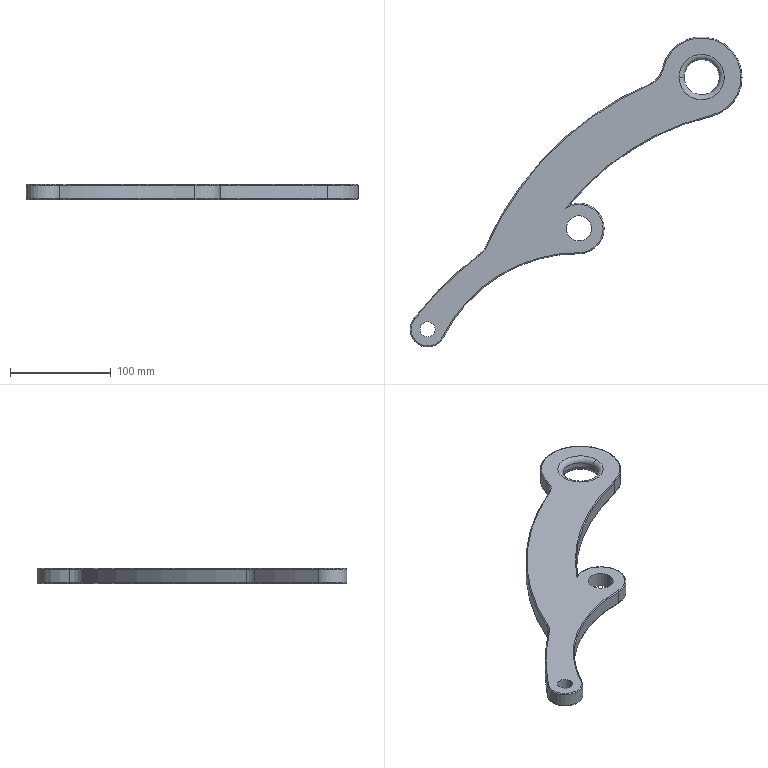Part | SolidWorks | features Fillet 3, HoleWzd 3, Extrusion 1 | 1 solid | 45 faces | box 329.193 x 307.5 x 15 mm | volume 313638 mm3 | torus 26 | cylinder 17 | plane 2 | commonest cylinder face diameters 35 x3 15 x2 25 x2 40 x2 50 x2 80 x2
STEP:
#1=CARTESIAN_POINT('',(254.193,250.,5.));
#2=VERTEX_POINT('',#1);
#3=CARTESIAN_POINT('',(289.193,250.,5.));
#4=VERTEX_POINT('',#3);
#5=CARTESIAN_POINT('',(271.693,250.,5.));
#6=DIRECTION('',(0.,0.,-1.));
#7=DIRECTION('',(1.,0.,0.));
#8=AXIS2_PLACEMENT_3D('',#5,#6,#7);
#9=CIRCLE('',#8,17.5);
#10=EDGE_CURVE('',#2,#4,#9,.T.);
#11=ORIENTED_EDGE('',*,*,#10,.F.);
#12=CARTESIAN_POINT('',(249.193,250.,0.));
#13=VERTEX_POINT('',#12);
#14=CARTESIAN_POINT('',(249.193,250.,5.));
#15=DIRECTION('',(0.,1.,0.));
#16=DIRECTION('',(-1.,0.,0.));
#17=AXIS2_PLACEMENT_3D('',#14,#15,#16);
#18=CIRCLE('',#17,5.);
#19=EDGE_CURVE('',#2,#13,#18,.T.);
#20=ORIENTED_EDGE('',*,*,#19,.T.);
#21=CARTESIAN_POINT('',(294.193,250.,0.));
#22=VERTEX_POINT('',#21);
#23=CARTESIAN_POINT('',(271.693,250.,0.));
#24=DIRECTION('',(0.,0.,1.));
#25=DIRECTION('',(1.,0.,0.));
#26=AXIS2_PLACEMENT_3D('',#23,#24,#25);
#27=CIRCLE('',#26,22.5);
#28=EDGE_CURVE('',#22,#13,#27,.T.);
#29=ORIENTED_EDGE('',*,*,#28,.F.);
#30=CARTESIAN_POINT('',(294.193,250.,5.));
#31=DIRECTION('',(0.,-1.,0.));
#32=DIRECTION('',(0.,0.,-1.));
#33=AXIS2_PLACEMENT_3D('',#30,#31,#32);
#34=CIRCLE('',#33,5.);
#35=EDGE_CURVE('',#4,#22,#34,.T.);
#36=ORIENTED_EDGE('',*,*,#35,.F.);
#37=EDGE_LOOP('',(#11,#20,#29,#36));
#38=FACE_OUTER_BOUND('',#37,.T.);
#39=CARTESIAN_POINT('',(271.693,250.,5.));
#40=DIRECTION('',(0.,0.,1.));
#41=DIRECTION('',(1.,0.,0.));
#42=AXIS2_PLACEMENT_3D('',#39,#40,#41);
#43=TOROIDAL_SURFACE('',#42,22.5,5.);
#44=ADVANCED_FACE('',(#38),#43,.T.);
#45=CARTESIAN_POINT('',(249.193,250.,15.));
#46=VERTEX_POINT('',#45);
#47=CARTESIAN_POINT('',(294.193,250.,15.));
#48=VERTEX_POINT('',#47);
#49=CARTESIAN_POINT('',(271.693,250.,15.));
#50=DIRECTION('',(0.,0.,-1.));
#51=DIRECTION('',(1.,0.,0.));
#52=AXIS2_PLACEMENT_3D('',#49,#50,#51);
#53=CIRCLE('',#52,22.5);
#54=EDGE_CURVE('',#46,#48,#53,.T.);
#55=ORIENTED_EDGE('',*,*,#54,.F.);
#56=CARTESIAN_POINT('',(254.193,250.,10.));
#57=VERTEX_POINT('',#56);
#58=CARTESIAN_POINT('',(249.193,250.,10.));
#59=DIRECTION('',(0.,1.,0.));
#60=DIRECTION('',(-1.,0.,0.));
#61=AXIS2_PLACEMENT_3D('',#58,#59,#60);
#62=CIRCLE('',#61,5.);
#63=EDGE_CURVE('',#46,#57,#62,.T.);
#64=ORIENTED_EDGE('',*,*,#63,.T.);
#65=CARTESIAN_POINT('',(289.193,250.,10.));
#66=VERTEX_POINT('',#65);
#67=CARTESIAN_POINT('',(271.693,250.,10.));
#68=DIRECTION('',(0.,0.,1.));
#69=DIRECTION('',(1.,0.,0.));
#70=AXIS2_PLACEMENT_3D('',#67,#68,#69);
#71=CIRCLE('',#70,17.5);
#72=EDGE_CURVE('',#66,#57,#71,.T.);
#73=ORIENTED_EDGE('',*,*,#72,.F.);
#74=CARTESIAN_POINT('',(294.193,250.,10.));
#75=DIRECTION('',(0.,-1.,0.));
#76=DIRECTION('',(0.,0.,-1.));
#77=AXIS2_PLACEMENT_3D('',#74,#75,#76);
#78=CIRCLE('',#77,5.);
#79=EDGE_CURVE('',#48,#66,#78,.T.);
#80=ORIENTED_EDGE('',*,*,#79,.F.);
#81=EDGE_LOOP('',(#55,#64,#73,#80));
#82=FACE_OUTER_BOUND('',#81,.T.);
#83=CARTESIAN_POINT('',(271.693,250.,10.));
#84=DIRECTION('',(0.,0.,1.));
#85=DIRECTION('',(1.,0.,0.));
#86=AXIS2_PLACEMENT_3D('',#83,#84,#85);
#87=TOROIDAL_SURFACE('',#86,22.5,5.);
#88=ADVANCED_FACE('',(#82),#87,.T.);
#89=CARTESIAN_POINT('',(311.693,250.,14.));
#90=VERTEX_POINT('',#89);
#91=CARTESIAN_POINT('',(281.029,211.105,14.));
#92=VERTEX_POINT('',#91);
#93=CARTESIAN_POINT('',(271.693,250.,14.));
#94=DIRECTION('',(0.,0.,-1.));
#95=DIRECTION('',(1.,0.,0.));
#96=AXIS2_PLACEMENT_3D('',#93,#94,#95);
#97=CIRCLE('',#96,40.);
#98=EDGE_CURVE('',#90,#92,#97,.T.);
#99=ORIENTED_EDGE('',*,*,#98,.F.);
#100=CARTESIAN_POINT('',(310.693,250.,15.));
#101=VERTEX_POINT('',#100);
#102=CARTESIAN_POINT('',(310.693,250.,14.));
#103=DIRECTION('',(0.,-1.,0.));
#104=DIRECTION('',(0.,0.,-1.));
#105=AXIS2_PLACEMENT_3D('',#102,#103,#104);
#106=CIRCLE('',#105,1.);
#107=EDGE_CURVE('',#90,#101,#106,.T.);
#108=ORIENTED_EDGE('',*,*,#107,.T.);
#109=CARTESIAN_POINT('',(280.795,212.077,15.));
#110=VERTEX_POINT('',#109);
#111=CARTESIAN_POINT('',(271.693,250.,15.));
#112=DIRECTION('',(0.,0.,1.));
#113=DIRECTION('',(1.,0.,0.));
#114=AXIS2_PLACEMENT_3D('',#111,#112,#113);
#115=CIRCLE('',#114,39.);
#116=EDGE_CURVE('',#110,#101,#115,.T.);
#117=ORIENTED_EDGE('',*,*,#116,.F.);
#118=CARTESIAN_POINT('',(280.795,212.077,14.));
#119=DIRECTION('',(-0.9724,-0.2334,0.));
#120=DIRECTION('',(0.2334,-0.9724,0.));
#121=AXIS2_PLACEMENT_3D('',#118,#119,#120);
#122=CIRCLE('',#121,1.);
#123=EDGE_CURVE('',#92,#110,#122,.T.);
#124=ORIENTED_EDGE('',*,*,#123,.F.);
#125=EDGE_LOOP('',(#99,#108,#117,#124));
#126=FACE_OUTER_BOUND('',#125,.T.);
#127=CARTESIAN_POINT('',(271.693,250.,14.));
#128=DIRECTION('',(0.,0.,1.));
#129=DIRECTION('',(1.,0.,0.));
#130=AXIS2_PLACEMENT_3D('',#127,#128,#129);
#131=TOROIDAL_SURFACE('',#130,39.,1.);
#132=ADVANCED_FACE('',(#126),#131,.T.);
#133=CARTESIAN_POINT('',(175.,100.,14.));
#134=VERTEX_POINT('',#133);
#135=CARTESIAN_POINT('',(149.967,75.,14.));
#136=VERTEX_POINT('',#135);
#137=CARTESIAN_POINT('',(150.,100.,14.));
#138=DIRECTION('',(0.,0.,-1.));
#139=DIRECTION('',(1.,0.,0.));
#140=AXIS2_PLACEMENT_3D('',#137,#138,#139);
#141=CIRCLE('',#140,25.);
#142=EDGE_CURVE('',#134,#136,#141,.T.);
#143=ORIENTED_EDGE('',*,*,#142,.F.);
#144=CARTESIAN_POINT('',(174.,100.,15.));
#145=VERTEX_POINT('',#144);
#146=CARTESIAN_POINT('',(174.,100.,14.));
#147=DIRECTION('',(0.,-1.,0.));
#148=DIRECTION('',(0.,0.,-1.));
#149=AXIS2_PLACEMENT_3D('',#146,#147,#148);
#150=CIRCLE('',#149,1.);
#151=EDGE_CURVE('',#134,#145,#150,.T.);
#152=ORIENTED_EDGE('',*,*,#151,.T.);
#153=CARTESIAN_POINT('',(149.969,76.,15.));
#154=VERTEX_POINT('',#153);
#155=CARTESIAN_POINT('',(150.,100.,15.));
#156=DIRECTION('',(0.,0.,1.));
#157=DIRECTION('',(1.,0.,0.));
#158=AXIS2_PLACEMENT_3D('',#155,#156,#157);
#159=CIRCLE('',#158,24.);
#160=EDGE_CURVE('',#154,#145,#159,.T.);
#161=ORIENTED_EDGE('',*,*,#160,.F.);
#162=CARTESIAN_POINT('',(149.969,76.,14.));
#163=DIRECTION('',(1.,-0.00131,0.));
#164=DIRECTION('',(0.00131,1.,0.));
#165=AXIS2_PLACEMENT_3D('',#162,#163,#164);
#166=CIRCLE('',#165,1.);
#167=EDGE_CURVE('',#154,#136,#166,.T.);
#168=ORIENTED_EDGE('',*,*,#167,.T.);
#169=EDGE_LOOP('',(#143,#152,#161,#168));
#170=FACE_OUTER_BOUND('',#169,.T.);
#171=CARTESIAN_POINT('',(150.,100.,14.));
#172=DIRECTION('',(0.,0.,1.));
#173=DIRECTION('',(1.,0.,0.));
#174=AXIS2_PLACEMENT_3D('',#171,#172,#173);
#175=TOROIDAL_SURFACE('',#174,24.,1.);
#176=ADVANCED_FACE('',(#170),#175,.T.);
#177=CARTESIAN_POINT('',(310.693,250.,0.));
#178=VERTEX_POINT('',#177);
#179=CARTESIAN_POINT('',(280.795,212.077,0.));
#180=VERTEX_POINT('',#179);
#181=CARTESIAN_POINT('',(271.693,250.,0.));
#182=DIRECTION('',(0.,0.,-1.));
#183=DIRECTION('',(1.,0.,0.));
#184=AXIS2_PLACEMENT_3D('',#181,#182,#183);
#185=CIRCLE('',#184,39.);
#186=EDGE_CURVE('',#178,#180,#185,.T.);
#187=ORIENTED_EDGE('',*,*,#186,.F.);
#188=CARTESIAN_POINT('',(311.693,250.,1.));
#189=VERTEX_POINT('',#188);
#190=CARTESIAN_POINT('',(310.693,250.,1.));
#191=DIRECTION('',(0.,-1.,0.));
#192=DIRECTION('',(0.,0.,-1.));
#193=AXIS2_PLACEMENT_3D('',#190,#191,#192);
#194=CIRCLE('',#193,1.);
#195=EDGE_CURVE('',#178,#189,#194,.T.);
#196=ORIENTED_EDGE('',*,*,#195,.T.);
#197=CARTESIAN_POINT('',(281.029,211.105,1.));
#198=VERTEX_POINT('',#197);
#199=CARTESIAN_POINT('',(271.693,250.,1.));
#200=DIRECTION('',(0.,0.,1.));
#201=DIRECTION('',(1.,0.,0.));
#202=AXIS2_PLACEMENT_3D('',#199,#200,#201);
#203=CIRCLE('',#202,40.);
#204=EDGE_CURVE('',#198,#189,#203,.T.);
#205=ORIENTED_EDGE('',*,*,#204,.F.);
#206=CARTESIAN_POINT('',(280.795,212.077,1.));
#207=DIRECTION('',(-0.9724,-0.2334,0.));
#208=DIRECTION('',(0.2334,-0.9724,0.));
#209=AXIS2_PLACEMENT_3D('',#206,#207,#208);
#210=CIRCLE('',#209,1.);
#211=EDGE_CURVE('',#180,#198,#210,.T.);
#212=ORIENTED_EDGE('',*,*,#211,.F.);
#213=EDGE_LOOP('',(#187,#196,#205,#212));
#214=FACE_OUTER_BOUND('',#213,.T.);
#215=CARTESIAN_POINT('',(271.693,250.,1.));
#216=DIRECTION('',(0.,0.,1.));
#217=DIRECTION('',(1.,0.,0.));
#218=AXIS2_PLACEMENT_3D('',#215,#216,#217);
#219=TOROIDAL_SURFACE('',#218,39.,1.);
#220=ADVANCED_FACE('',(#214),#219,.T.);
#221=CARTESIAN_POINT('',(174.,100.,0.));
#222=VERTEX_POINT('',#221);
#223=CARTESIAN_POINT('',(149.969,76.,0.));
#224=VERTEX_POINT('',#223);
#225=CARTESIAN_POINT('',(150.,100.,0.));
#226=DIRECTION('',(0.,0.,-1.));
#227=DIRECTION('',(1.,0.,0.));
#228=AXIS2_PLACEMENT_3D('',#225,#226,#227);
#229=CIRCLE('',#228,24.);
#230=EDGE_CURVE('',#222,#224,#229,.T.);
#231=ORIENTED_EDGE('',*,*,#230,.F.);
#232=CARTESIAN_POINT('',(175.,100.,1.));
#233=VERTEX_POINT('',#232);
#234=CARTESIAN_POINT('',(174.,100.,1.));
#235=DIRECTION('',(0.,-1.,0.));
#236=DIRECTION('',(0.,0.,-1.));
#237=AXIS2_PLACEMENT_3D('',#234,#235,#236);
#238=CIRCLE('',#237,1.);
#239=EDGE_CURVE('',#222,#233,#238,.T.);
#240=ORIENTED_EDGE('',*,*,#239,.T.);
#241=CARTESIAN_POINT('',(149.967,75.,1.));
#242=VERTEX_POINT('',#241);
#243=CARTESIAN_POINT('',(150.,100.,1.));
#244=DIRECTION('',(0.,0.,1.));
#245=DIRECTION('',(1.,0.,0.));
#246=AXIS2_PLACEMENT_3D('',#243,#244,#245);
#247=CIRCLE('',#246,25.);
#248=EDGE_CURVE('',#242,#233,#247,.T.);
#249=ORIENTED_EDGE('',*,*,#248,.F.);
#250=CARTESIAN_POINT('',(149.969,76.,1.));
#251=DIRECTION('',(1.,-0.00131,0.));
#252=DIRECTION('',(0.00131,1.,0.));
#253=AXIS2_PLACEMENT_3D('',#250,#251,#252);
#254=CIRCLE('',#253,1.);
#255=EDGE_CURVE('',#242,#224,#254,.T.);
#256=ORIENTED_EDGE('',*,*,#255,.T.);
#257=EDGE_LOOP('',(#231,#240,#249,#256));
#258=FACE_OUTER_BOUND('',#257,.T.);
#259=CARTESIAN_POINT('',(150.,100.,1.));
#260=DIRECTION('',(0.,0.,1.));
#261=DIRECTION('',(1.,0.,0.));
#262=AXIS2_PLACEMENT_3D('',#259,#260,#261);
#263=TOROIDAL_SURFACE('',#262,24.,1.);
#264=ADVANCED_FACE('',(#258),#263,.T.);
#265=CARTESIAN_POINT('',(7.5,0.,15.));
#266=VERTEX_POINT('',#265);
#267=CARTESIAN_POINT('',(-7.5,0.,15.));
#268=VERTEX_POINT('',#267);
#269=CARTESIAN_POINT('',(0.,0.,15.));
#270=DIRECTION('',(0.,0.,-1.));
#271=DIRECTION('',(-1.,0.,0.));
#272=AXIS2_PLACEMENT_3D('',#269,#270,#271);
#273=CIRCLE('',#272,7.5);
#274=EDGE_CURVE('',#266,#268,#273,.T.);
#275=ORIENTED_EDGE('',*,*,#274,.F.);
#276=CARTESIAN_POINT('',(7.5,0.,0.));
#277=VERTEX_POINT('',#276);
#278=CARTESIAN_POINT('',(7.5,0.,0.));
#279=DIRECTION('',(0.,0.,-1.));
#280=VECTOR('',#279,1000.);
#281=LINE('',#278,#280);
#282=EDGE_CURVE('',#266,#277,#281,.T.);
#283=ORIENTED_EDGE('',*,*,#282,.T.);
#284=CARTESIAN_POINT('',(-7.5,0.,0.));
#285=VERTEX_POINT('',#284);
#286=CARTESIAN_POINT('',(0.,0.,0.));
#287=DIRECTION('',(0.,0.,-1.));
#288=DIRECTION('',(-1.,0.,0.));
#289=AXIS2_PLACEMENT_3D('',#286,#287,#288);
#290=CIRCLE('',#289,7.5);
#291=EDGE_CURVE('',#277,#285,#290,.T.);
#292=ORIENTED_EDGE('',*,*,#291,.T.);
#293=CARTESIAN_POINT('',(-7.5,0.,0.));
#294=DIRECTION('',(0.,0.,-1.));
#295=VECTOR('',#294,1000.);
#296=LINE('',#293,#295);
#297=EDGE_CURVE('',#268,#285,#296,.T.);
#298=ORIENTED_EDGE('',*,*,#297,.F.);
#299=EDGE_LOOP('',(#275,#283,#292,#298));
#300=FACE_OUTER_BOUND('',#299,.T.);
#301=CARTESIAN_POINT('',(0.,0.,0.));
#302=DIRECTION('',(0.,0.,-1.));
#303=DIRECTION('',(-1.,0.,0.));
#304=AXIS2_PLACEMENT_3D('',#301,#302,#303);
#305=CYLINDRICAL_SURFACE('',#304,7.5);
#306=ADVANCED_FACE('',(#300),#305,.F.);
#307=CARTESIAN_POINT('',(162.5,100.,15.));
#308=VERTEX_POINT('',#307);
#309=CARTESIAN_POINT('',(137.5,100.,15.));
#310=VERTEX_POINT('',#309);
#311=CARTESIAN_POINT('',(150.,100.,15.));
#312=DIRECTION('',(0.,0.,-1.));
#313=DIRECTION('',(-1.,0.,0.));
#314=AXIS2_PLACEMENT_3D('',#311,#312,#313);
#315=CIRCLE('',#314,12.5);
#316=EDGE_CURVE('',#308,#310,#315,.T.);
#317=ORIENTED_EDGE('',*,*,#316,.F.);
#318=CARTESIAN_POINT('',(162.5,100.,0.));
#319=VERTEX_POINT('',#318);
#320=CARTESIAN_POINT('',(162.5,100.,0.));
#321=DIRECTION('',(0.,0.,-1.));
#322=VECTOR('',#321,1000.);
#323=LINE('',#320,#322);
#324=EDGE_CURVE('',#308,#319,#323,.T.);
#325=ORIENTED_EDGE('',*,*,#324,.T.);
#326=CARTESIAN_POINT('',(137.5,100.,0.));
#327=VERTEX_POINT('',#326);
#328=CARTESIAN_POINT('',(150.,100.,0.));
#329=DIRECTION('',(0.,0.,-1.));
#330=DIRECTION('',(-1.,0.,0.));
#331=AXIS2_PLACEMENT_3D('',#328,#329,#330);
#332=CIRCLE('',#331,12.5);
#333=EDGE_CURVE('',#319,#327,#332,.T.);
#334=ORIENTED_EDGE('',*,*,#333,.T.);
#335=CARTESIAN_POINT('',(137.5,100.,0.));
#336=DIRECTION('',(0.,0.,-1.));
#337=VECTOR('',#336,1000.);
#338=LINE('',#335,#337);
#339=EDGE_CURVE('',#310,#327,#338,.T.);
#340=ORIENTED_EDGE('',*,*,#339,.F.);
#341=EDGE_LOOP('',(#317,#325,#334,#340));
#342=FACE_OUTER_BOUND('',#341,.T.);
#343=CARTESIAN_POINT('',(150.,100.,0.));
#344=DIRECTION('',(0.,0.,-1.));
#345=DIRECTION('',(-1.,0.,0.));
#346=AXIS2_PLACEMENT_3D('',#343,#344,#345);
#347=CYLINDRICAL_SURFACE('',#346,12.5);
#348=ADVANCED_FACE('',(#342),#347,.F.);
#349=CARTESIAN_POINT('',(271.693,250.,10.));
#350=DIRECTION('',(0.,0.,1.));
#351=DIRECTION('',(1.,0.,0.));
#352=AXIS2_PLACEMENT_3D('',#349,#350,#351);
#353=CIRCLE('',#352,17.5);
#354=EDGE_CURVE('',#57,#66,#353,.T.);
#355=ORIENTED_EDGE('',*,*,#354,.T.);
#356=CARTESIAN_POINT('',(289.193,250.,0.));
#357=DIRECTION('',(0.,0.,-1.));
#358=VECTOR('',#357,1000.);
#359=LINE('',#356,#358);
#360=EDGE_CURVE('',#66,#4,#359,.T.);
#361=ORIENTED_EDGE('',*,*,#360,.T.);
#362=CARTESIAN_POINT('',(271.693,250.,5.));
#363=DIRECTION('',(0.,0.,-1.));
#364=DIRECTION('',(1.,0.,0.));
#365=AXIS2_PLACEMENT_3D('',#362,#363,#364);
#366=CIRCLE('',#365,17.5);
#367=EDGE_CURVE('',#4,#2,#366,.T.);
#368=ORIENTED_EDGE('',*,*,#367,.T.);
#369=CARTESIAN_POINT('',(254.193,250.,0.));
#370=DIRECTION('',(0.,0.,-1.));
#371=VECTOR('',#370,1000.);
#372=LINE('',#369,#371);
#373=EDGE_CURVE('',#57,#2,#372,.T.);
#374=ORIENTED_EDGE('',*,*,#373,.F.);
#375=EDGE_LOOP('',(#355,#361,#368,#374));
#376=FACE_OUTER_BOUND('',#375,.T.);
#377=CARTESIAN_POINT('',(271.693,250.,0.));
#378=DIRECTION('',(0.,0.,-1.));
#379=DIRECTION('',(-1.,0.,0.));
#380=AXIS2_PLACEMENT_3D('',#377,#378,#379);
#381=CYLINDRICAL_SURFACE('',#380,17.5);
#382=ADVANCED_FACE('',(#376),#381,.F.);
#383=ORIENTED_EDGE('',*,*,#248,.T.);
#384=CARTESIAN_POINT('',(175.,100.,0.));
#385=DIRECTION('',(0.,0.,1.));
#386=VECTOR('',#385,1000.);
#387=LINE('',#384,#386);
#388=EDGE_CURVE('',#233,#134,#387,.T.);
#389=ORIENTED_EDGE('',*,*,#388,.T.);
#390=ORIENTED_EDGE('',*,*,#142,.T.);
#391=CARTESIAN_POINT('',(149.967,75.,0.));
#392=DIRECTION('',(0.,0.,1.));
#393=VECTOR('',#392,1000.);
#394=LINE('',#391,#393);
#395=EDGE_CURVE('',#242,#136,#394,.T.);
#396=ORIENTED_EDGE('',*,*,#395,.F.);
#397=EDGE_LOOP('',(#383,#389,#390,#396));
#398=FACE_OUTER_BOUND('',#397,.T.);
#399=CARTESIAN_POINT('',(150.,100.,0.));
#400=DIRECTION('',(0.,0.,1.));
#401=DIRECTION('',(1.,0.,0.));
#402=AXIS2_PLACEMENT_3D('',#399,#400,#401);
#403=CYLINDRICAL_SURFACE('',#402,25.);
#404=ADVANCED_FACE('',(#398),#403,.T.);
#405=ORIENTED_EDGE('',*,*,#204,.T.);
#406=CARTESIAN_POINT('',(311.693,250.,0.));
#407=DIRECTION('',(0.,0.,1.));
#408=VECTOR('',#407,1000.);
#409=LINE('',#406,#408);
#410=EDGE_CURVE('',#189,#90,#409,.T.);
#411=ORIENTED_EDGE('',*,*,#410,.T.);
#412=ORIENTED_EDGE('',*,*,#98,.T.);
#413=CARTESIAN_POINT('',(281.029,211.105,0.));
#414=DIRECTION('',(0.,0.,1.));
#415=VECTOR('',#414,1000.);
#416=LINE('',#413,#415);
#417=EDGE_CURVE('',#198,#92,#416,.T.);
#418=ORIENTED_EDGE('',*,*,#417,.F.);
#419=EDGE_LOOP('',(#405,#411,#412,#418));
#420=FACE_OUTER_BOUND('',#419,.T.);
#421=CARTESIAN_POINT('',(271.693,250.,0.));
#422=DIRECTION('',(0.,0.,1.));
#423=DIRECTION('',(1.,0.,0.));
#424=AXIS2_PLACEMENT_3D('',#421,#422,#423);
#425=CYLINDRICAL_SURFACE('',#424,40.);
#426=ADVANCED_FACE('',(#420),#425,.T.);
#427=ORIENTED_EDGE('',*,*,#410,.F.);
#428=CARTESIAN_POINT('',(232.517,258.08,1.));
#429=VERTEX_POINT('',#428);
#430=CARTESIAN_POINT('',(271.693,250.,1.));
#431=DIRECTION('',(0.,0.,1.));
#432=DIRECTION('',(1.,0.,0.));
#433=AXIS2_PLACEMENT_3D('',#430,#431,#432);
#434=CIRCLE('',#433,40.);
#435=EDGE_CURVE('',#189,#429,#434,.T.);
#436=ORIENTED_EDGE('',*,*,#435,.T.);
#437=CARTESIAN_POINT('',(232.517,258.08,14.));
#438=VERTEX_POINT('',#437);
#439=CARTESIAN_POINT('',(232.517,258.08,0.));
#440=DIRECTION('',(0.,0.,1.));
#441=VECTOR('',#440,1000.);
#442=LINE('',#439,#441);
#443=EDGE_CURVE('',#429,#438,#442,.T.);
#444=ORIENTED_EDGE('',*,*,#443,.T.);
#445=CARTESIAN_POINT('',(271.693,250.,14.));
#446=DIRECTION('',(0.,0.,-1.));
#447=DIRECTION('',(1.,0.,0.));
#448=AXIS2_PLACEMENT_3D('',#445,#446,#447);
#449=CIRCLE('',#448,40.);
#450=EDGE_CURVE('',#438,#90,#449,.T.);
#451=ORIENTED_EDGE('',*,*,#450,.T.);
#452=EDGE_LOOP('',(#427,#436,#444,#451));
#453=FACE_OUTER_BOUND('',#452,.T.);
#454=CARTESIAN_POINT('',(271.693,250.,0.));
#455=DIRECTION('',(0.,0.,1.));
#456=DIRECTION('',(1.,0.,0.));
#457=AXIS2_PLACEMENT_3D('',#454,#455,#456);
#458=CYLINDRICAL_SURFACE('',#457,40.);
#459=ADVANCED_FACE('',(#453),#458,.T.);
#460=CARTESIAN_POINT('',(140.715,123.212,1.));
#461=VERTEX_POINT('',#460);
#462=CARTESIAN_POINT('',(140.715,123.212,14.));
#463=VERTEX_POINT('',#462);
#464=CARTESIAN_POINT('',(140.715,123.212,0.));
#465=DIRECTION('',(0.,0.,1.));
#466=VECTOR('',#465,1000.);
#467=LINE('',#464,#466);
#468=EDGE_CURVE('',#461,#463,#467,.T.);
#469=ORIENTED_EDGE('',*,*,#468,.F.);
#470=CARTESIAN_POINT('',(341.711,-41.715,1.));
#471=DIRECTION('',(0.,0.,-1.));
#472=DIRECTION('',(1.,0.,0.));
#473=AXIS2_PLACEMENT_3D('',#470,#471,#472);
#474=CIRCLE('',#473,260.);
#475=EDGE_CURVE('',#461,#198,#474,.T.);
#476=ORIENTED_EDGE('',*,*,#475,.T.);
#477=ORIENTED_EDGE('',*,*,#417,.T.);
#478=CARTESIAN_POINT('',(341.711,-41.715,14.));
#479=DIRECTION('',(0.,0.,1.));
#480=DIRECTION('',(1.,0.,0.));
#481=AXIS2_PLACEMENT_3D('',#478,#479,#480);
#482=CIRCLE('',#481,260.);
#483=EDGE_CURVE('',#92,#463,#482,.T.);
#484=ORIENTED_EDGE('',*,*,#483,.T.);
#485=EDGE_LOOP('',(#469,#476,#477,#484));
#486=FACE_OUTER_BOUND('',#485,.T.);
#487=CARTESIAN_POINT('',(341.711,-41.715,0.));
#488=DIRECTION('',(0.,0.,1.));
#489=DIRECTION('',(1.,0.,0.));
#490=AXIS2_PLACEMENT_3D('',#487,#488,#489);
#491=CYLINDRICAL_SURFACE('',#490,260.);
#492=ADVANCED_FACE('',(#486),#491,.F.);
#493=ORIENTED_EDGE('',*,*,#388,.F.);
#494=CARTESIAN_POINT('',(150.,100.,1.));
#495=DIRECTION('',(0.,0.,1.));
#496=DIRECTION('',(1.,0.,0.));
#497=AXIS2_PLACEMENT_3D('',#494,#495,#496);
#498=CIRCLE('',#497,25.);
#499=EDGE_CURVE('',#233,#461,#498,.T.);
#500=ORIENTED_EDGE('',*,*,#499,.T.);
#501=ORIENTED_EDGE('',*,*,#468,.T.);
#502=CARTESIAN_POINT('',(150.,100.,14.));
#503=DIRECTION('',(0.,0.,-1.));
#504=DIRECTION('',(1.,0.,0.));
#505=AXIS2_PLACEMENT_3D('',#502,#503,#504);
#506=CIRCLE('',#505,25.);
#507=EDGE_CURVE('',#463,#134,#506,.T.);
#508=ORIENTED_EDGE('',*,*,#507,.T.);
#509=EDGE_LOOP('',(#493,#500,#501,#508));
#510=FACE_OUTER_BOUND('',#509,.T.);
#511=CARTESIAN_POINT('',(150.,100.,0.));
#512=DIRECTION('',(0.,0.,1.));
#513=DIRECTION('',(1.,0.,0.));
#514=AXIS2_PLACEMENT_3D('',#511,#512,#513);
#515=CYLINDRICAL_SURFACE('',#514,25.);
#516=ADVANCED_FACE('',(#510),#515,.T.);
#517=CARTESIAN_POINT('',(15.648,-7.836,1.));
#518=VERTEX_POINT('',#517);
#519=CARTESIAN_POINT('',(15.648,-7.836,14.));
#520=VERTEX_POINT('',#519);
#521=CARTESIAN_POINT('',(15.648,-7.836,0.));
#522=DIRECTION('',(0.,0.,1.));
#523=VECTOR('',#522,1000.);
#524=LINE('',#521,#523);
#525=EDGE_CURVE('',#518,#520,#524,.T.);
#526=ORIENTED_EDGE('',*,*,#525,.F.);
#527=CARTESIAN_POINT('',(149.771,-75.,1.));
#528=DIRECTION('',(0.,0.,-1.));
#529=DIRECTION('',(1.,0.,0.));
#530=AXIS2_PLACEMENT_3D('',#527,#528,#529);
#531=CIRCLE('',#530,150.);
#532=EDGE_CURVE('',#518,#242,#531,.T.);
#533=ORIENTED_EDGE('',*,*,#532,.T.);
#534=ORIENTED_EDGE('',*,*,#395,.T.);
#535=CARTESIAN_POINT('',(149.771,-75.,14.));
#536=DIRECTION('',(0.,0.,1.));
#537=DIRECTION('',(1.,0.,0.));
#538=AXIS2_PLACEMENT_3D('',#535,#536,#537);
#539=CIRCLE('',#538,150.);
#540=EDGE_CURVE('',#136,#520,#539,.T.);
#541=ORIENTED_EDGE('',*,*,#540,.T.);
#542=EDGE_LOOP('',(#526,#533,#534,#541));
#543=FACE_OUTER_BOUND('',#542,.T.);
#544=CARTESIAN_POINT('',(149.771,-75.,0.));
#545=DIRECTION('',(0.,0.,1.));
#546=DIRECTION('',(1.,0.,0.));
#547=AXIS2_PLACEMENT_3D('',#544,#545,#546);
#548=CYLINDRICAL_SURFACE('',#547,150.);
#549=ADVANCED_FACE('',(#543),#548,.F.);
#550=CARTESIAN_POINT('',(-13.768,10.803,1.));
#551=VERTEX_POINT('',#550);
#552=CARTESIAN_POINT('',(-13.768,10.803,14.));
#553=VERTEX_POINT('',#552);
#554=CARTESIAN_POINT('',(-13.768,10.803,0.));
#555=DIRECTION('',(0.,0.,1.));
#556=VECTOR('',#555,1000.);
#557=LINE('',#554,#556);
#558=EDGE_CURVE('',#551,#553,#557,.T.);
#559=ORIENTED_EDGE('',*,*,#558,.F.);
#560=CARTESIAN_POINT('',(0.,0.,1.));
#561=DIRECTION('',(0.,0.,1.));
#562=DIRECTION('',(1.,0.,0.));
#563=AXIS2_PLACEMENT_3D('',#560,#561,#562);
#564=CIRCLE('',#563,17.5);
#565=EDGE_CURVE('',#551,#518,#564,.T.);
#566=ORIENTED_EDGE('',*,*,#565,.T.);
#567=ORIENTED_EDGE('',*,*,#525,.T.);
#568=CARTESIAN_POINT('',(0.,0.,14.));
#569=DIRECTION('',(0.,0.,-1.));
#570=DIRECTION('',(1.,0.,0.));
#571=AXIS2_PLACEMENT_3D('',#568,#569,#570);
#572=CIRCLE('',#571,17.5);
#573=EDGE_CURVE('',#520,#553,#572,.T.);
#574=ORIENTED_EDGE('',*,*,#573,.T.);
#575=EDGE_LOOP('',(#559,#566,#567,#574));
#576=FACE_OUTER_BOUND('',#575,.T.);
#577=CARTESIAN_POINT('',(0.,0.,0.));
#578=DIRECTION('',(0.,0.,1.));
#579=DIRECTION('',(1.,0.,0.));
#580=AXIS2_PLACEMENT_3D('',#577,#578,#579);
#581=CYLINDRICAL_SURFACE('',#580,17.5);
#582=ADVANCED_FACE('',(#576),#581,.T.);
#583=CARTESIAN_POINT('',(51.411,74.615,14.));
#584=VERTEX_POINT('',#583);
#585=CARTESIAN_POINT('',(51.411,74.615,1.));
#586=VERTEX_POINT('',#585);
#587=CARTESIAN_POINT('',(51.411,74.615,0.));
#588=DIRECTION('',(0.,0.,-1.));
#589=VECTOR('',#588,1000.);
#590=LINE('',#587,#589);
#591=EDGE_CURVE('',#584,#586,#590,.T.);
#592=ORIENTED_EDGE('',*,*,#591,.T.);
#593=CARTESIAN_POINT('',(261.585,-205.255,1.));
#594=DIRECTION('',(0.,0.,1.));
#595=DIRECTION('',(1.,0.,0.));
#596=AXIS2_PLACEMENT_3D('',#593,#594,#595);
#597=CIRCLE('',#596,350.);
#598=EDGE_CURVE('',#586,#551,#597,.T.);
#599=ORIENTED_EDGE('',*,*,#598,.T.);
#600=ORIENTED_EDGE('',*,*,#558,.T.);
#601=CARTESIAN_POINT('',(261.585,-205.255,14.));
#602=DIRECTION('',(0.,0.,-1.));
#603=DIRECTION('',(1.,0.,0.));
#604=AXIS2_PLACEMENT_3D('',#601,#602,#603);
#605=CIRCLE('',#604,350.);
#606=EDGE_CURVE('',#553,#584,#605,.T.);
#607=ORIENTED_EDGE('',*,*,#606,.T.);
#608=EDGE_LOOP('',(#592,#599,#600,#607));
#609=FACE_OUTER_BOUND('',#608,.T.);
#610=CARTESIAN_POINT('',(261.585,-205.255,0.));
#611=DIRECTION('',(0.,0.,1.));
#612=DIRECTION('',(1.,0.,0.));
#613=AXIS2_PLACEMENT_3D('',#610,#611,#612);
#614=CYLINDRICAL_SURFACE('',#613,350.);
#615=ADVANCED_FACE('',(#609),#614,.T.);
#616=CARTESIAN_POINT('',(220.735,243.706,14.));
#617=VERTEX_POINT('',#616);
#618=CARTESIAN_POINT('',(220.735,243.706,1.));
#619=VERTEX_POINT('',#618);
#620=CARTESIAN_POINT('',(220.735,243.706,0.));
#621=DIRECTION('',(0.,0.,-1.));
#622=VECTOR('',#621,1000.);
#623=LINE('',#620,#622);
#624=EDGE_CURVE('',#617,#619,#623,.T.);
#625=ORIENTED_EDGE('',*,*,#624,.T.);
#626=CARTESIAN_POINT('',(57.723,82.588,1.));
#627=VERTEX_POINT('',#626);
#628=CARTESIAN_POINT('',(341.711,-41.715,1.));
#629=DIRECTION('',(0.,0.,1.));
#630=DIRECTION('',(1.,0.,0.));
#631=AXIS2_PLACEMENT_3D('',#628,#629,#630);
#632=CIRCLE('',#631,310.);
#633=EDGE_CURVE('',#619,#627,#632,.T.);
#634=ORIENTED_EDGE('',*,*,#633,.T.);
#635=CARTESIAN_POINT('',(57.723,82.588,14.));
#636=VERTEX_POINT('',#635);
#637=CARTESIAN_POINT('',(57.723,82.588,0.));
#638=DIRECTION('',(0.,0.,1.));
#639=VECTOR('',#638,1000.);
#640=LINE('',#637,#639);
#641=EDGE_CURVE('',#627,#636,#640,.T.);
#642=ORIENTED_EDGE('',*,*,#641,.T.);
#643=CARTESIAN_POINT('',(341.711,-41.715,14.));
#644=DIRECTION('',(0.,0.,-1.));
#645=DIRECTION('',(1.,0.,0.));
#646=AXIS2_PLACEMENT_3D('',#643,#644,#645);
#647=CIRCLE('',#646,310.);
#648=EDGE_CURVE('',#636,#617,#647,.T.);
#649=ORIENTED_EDGE('',*,*,#648,.T.);
#650=EDGE_LOOP('',(#625,#634,#642,#649));
#651=FACE_OUTER_BOUND('',#650,.T.);
#652=CARTESIAN_POINT('',(341.711,-41.715,0.));
#653=DIRECTION('',(0.,0.,1.));
#654=DIRECTION('',(1.,0.,0.));
#655=AXIS2_PLACEMENT_3D('',#652,#653,#654);
#656=CYLINDRICAL_SURFACE('',#655,310.);
#657=ADVANCED_FACE('',(#651),#656,.T.);
#658=ORIENTED_EDGE('',*,*,#28,.T.);
#659=CARTESIAN_POINT('',(271.693,250.,0.));
#660=DIRECTION('',(0.,0.,1.));
#661=DIRECTION('',(1.,0.,0.));
#662=AXIS2_PLACEMENT_3D('',#659,#660,#661);
#663=CIRCLE('',#662,22.5);
#664=EDGE_CURVE('',#13,#22,#663,.T.);
#665=ORIENTED_EDGE('',*,*,#664,.T.);
#666=EDGE_LOOP('',(#658,#665));
#667=FACE_BOUND('',#666,.T.);
#668=CARTESIAN_POINT('',(233.497,257.878,0.));
#669=VERTEX_POINT('',#668);
#670=CARTESIAN_POINT('',(271.693,250.,0.));
#671=DIRECTION('',(0.,0.,-1.));
#672=DIRECTION('',(1.,0.,0.));
#673=AXIS2_PLACEMENT_3D('',#670,#671,#672);
#674=CIRCLE('',#673,39.);
#675=EDGE_CURVE('',#669,#178,#674,.T.);
#676=ORIENTED_EDGE('',*,*,#675,.T.);
#677=ORIENTED_EDGE('',*,*,#186,.T.);
#678=CARTESIAN_POINT('',(136.968,120.153,0.));
#679=VERTEX_POINT('',#678);
#680=CARTESIAN_POINT('',(341.711,-41.715,0.));
#681=DIRECTION('',(0.,0.,1.));
#682=DIRECTION('',(1.,0.,0.));
#683=AXIS2_PLACEMENT_3D('',#680,#681,#682);
#684=CIRCLE('',#683,261.);
#685=EDGE_CURVE('',#180,#679,#684,.T.);
#686=ORIENTED_EDGE('',*,*,#685,.T.);
#687=CARTESIAN_POINT('',(150.,100.,0.));
#688=DIRECTION('',(0.,0.,-1.));
#689=DIRECTION('',(1.,0.,0.));
#690=AXIS2_PLACEMENT_3D('',#687,#688,#689);
#691=CIRCLE('',#690,24.);
#692=EDGE_CURVE('',#679,#222,#691,.T.);
#693=ORIENTED_EDGE('',*,*,#692,.T.);
#694=ORIENTED_EDGE('',*,*,#230,.T.);
#695=CARTESIAN_POINT('',(14.754,-7.388,0.));
#696=VERTEX_POINT('',#695);
#697=CARTESIAN_POINT('',(149.771,-75.,0.));
#698=DIRECTION('',(0.,0.,1.));
#699=DIRECTION('',(1.,0.,0.));
#700=AXIS2_PLACEMENT_3D('',#697,#698,#699);
#701=CIRCLE('',#700,151.);
#702=EDGE_CURVE('',#224,#696,#701,.T.);
#703=ORIENTED_EDGE('',*,*,#702,.T.);
#704=CARTESIAN_POINT('',(-12.981,10.186,0.));
#705=VERTEX_POINT('',#704);
#706=CARTESIAN_POINT('',(0.,0.,0.));
#707=DIRECTION('',(0.,0.,-1.));
#708=DIRECTION('',(1.,0.,0.));
#709=AXIS2_PLACEMENT_3D('',#706,#707,#708);
#710=CIRCLE('',#709,16.5);
#711=EDGE_CURVE('',#696,#705,#710,.T.);
#712=ORIENTED_EDGE('',*,*,#711,.T.);
#713=CARTESIAN_POINT('',(52.012,73.815,0.));
#714=VERTEX_POINT('',#713);
#715=CARTESIAN_POINT('',(261.585,-205.255,0.));
#716=DIRECTION('',(0.,0.,-1.));
#717=DIRECTION('',(1.,0.,0.));
#718=AXIS2_PLACEMENT_3D('',#715,#716,#717);
#719=CIRCLE('',#718,349.);
#720=EDGE_CURVE('',#705,#714,#719,.T.);
#721=ORIENTED_EDGE('',*,*,#720,.T.);
#722=CARTESIAN_POINT('',(58.639,82.187,0.));
#723=VERTEX_POINT('',#722);
#724=CARTESIAN_POINT('',(39.402,90.607,0.));
#725=DIRECTION('',(0.,0.,1.));
#726=DIRECTION('',(1.,0.,0.));
#727=AXIS2_PLACEMENT_3D('',#724,#725,#726);
#728=CIRCLE('',#727,21.);
#729=EDGE_CURVE('',#714,#723,#728,.T.);
#730=ORIENTED_EDGE('',*,*,#729,.T.);
#731=CARTESIAN_POINT('',(221.125,242.785,0.));
#732=VERTEX_POINT('',#731);
#733=CARTESIAN_POINT('',(341.711,-41.715,0.));
#734=DIRECTION('',(0.,0.,-1.));
#735=DIRECTION('',(1.,0.,0.));
#736=AXIS2_PLACEMENT_3D('',#733,#734,#735);
#737=CIRCLE('',#736,309.);
#738=EDGE_CURVE('',#723,#732,#737,.T.);
#739=ORIENTED_EDGE('',*,*,#738,.T.);
#740=CARTESIAN_POINT('',(212.93,262.12,0.));
#741=DIRECTION('',(0.,0.,1.));
#742=DIRECTION('',(1.,0.,0.));
#743=AXIS2_PLACEMENT_3D('',#740,#741,#742);
#744=CIRCLE('',#743,21.);
#745=EDGE_CURVE('',#732,#669,#744,.T.);
#746=ORIENTED_EDGE('',*,*,#745,.T.);
#747=EDGE_LOOP('',(#676,#677,#686,#693,#694,#703,#712,#721,#730,#739,#746));
#748=FACE_OUTER_BOUND('',#747,.T.);
#749=CARTESIAN_POINT('',(0.,0.,0.));
#750=DIRECTION('',(0.,0.,-1.));
#751=DIRECTION('',(-1.,0.,0.));
#752=AXIS2_PLACEMENT_3D('',#749,#750,#751);
#753=CIRCLE('',#752,7.5);
#754=EDGE_CURVE('',#285,#277,#753,.T.);
#755=ORIENTED_EDGE('',*,*,#754,.F.);
#756=ORIENTED_EDGE('',*,*,#291,.F.);
#757=EDGE_LOOP('',(#755,#756));
#758=FACE_BOUND('',#757,.T.);
#759=CARTESIAN_POINT('',(150.,100.,0.));
#760=DIRECTION('',(0.,0.,-1.));
#761=DIRECTION('',(-1.,0.,0.));
#762=AXIS2_PLACEMENT_3D('',#759,#760,#761);
#763=CIRCLE('',#762,12.5);
#764=EDGE_CURVE('',#327,#319,#763,.T.);
#765=ORIENTED_EDGE('',*,*,#764,.F.);
#766=ORIENTED_EDGE('',*,*,#333,.F.);
#767=EDGE_LOOP('',(#765,#766));
#768=FACE_BOUND('',#767,.T.);
#769=CARTESIAN_POINT('',(306.702,104.143,0.));
#770=DIRECTION('',(0.,0.,1.));
#771=DIRECTION('',(1.,0.,0.));
#772=AXIS2_PLACEMENT_3D('',#769,#770,#771);
#773=PLANE('',#772);
#774=ADVANCED_FACE('',(#667,#748,#758,#768),#773,.F.);
#775=CARTESIAN_POINT('',(271.693,250.,15.));
#776=DIRECTION('',(0.,0.,-1.));
#777=DIRECTION('',(1.,0.,0.));
#778=AXIS2_PLACEMENT_3D('',#775,#776,#777);
#779=CIRCLE('',#778,22.5);
#780=EDGE_CURVE('',#48,#46,#779,.T.);
#781=ORIENTED_EDGE('',*,*,#780,.T.);
#782=ORIENTED_EDGE('',*,*,#54,.T.);
#783=EDGE_LOOP('',(#781,#782));
#784=FACE_BOUND('',#783,.T.);
#785=ORIENTED_EDGE('',*,*,#160,.T.);
#786=CARTESIAN_POINT('',(136.968,120.153,15.));
#787=VERTEX_POINT('',#786);
#788=CARTESIAN_POINT('',(150.,100.,15.));
#789=DIRECTION('',(0.,0.,1.));
#790=DIRECTION('',(1.,0.,0.));
#791=AXIS2_PLACEMENT_3D('',#788,#789,#790);
#792=CIRCLE('',#791,24.);
#793=EDGE_CURVE('',#145,#787,#792,.T.);
#794=ORIENTED_EDGE('',*,*,#793,.T.);
#795=CARTESIAN_POINT('',(341.711,-41.715,15.));
#796=DIRECTION('',(0.,0.,-1.));
#797=DIRECTION('',(1.,0.,0.));
#798=AXIS2_PLACEMENT_3D('',#795,#796,#797);
#799=CIRCLE('',#798,261.);
#800=EDGE_CURVE('',#787,#110,#799,.T.);
#801=ORIENTED_EDGE('',*,*,#800,.T.);
#802=ORIENTED_EDGE('',*,*,#116,.T.);
#803=CARTESIAN_POINT('',(233.497,257.878,15.));
#804=VERTEX_POINT('',#803);
#805=CARTESIAN_POINT('',(271.693,250.,15.));
#806=DIRECTION('',(0.,0.,1.));
#807=DIRECTION('',(1.,0.,0.));
#808=AXIS2_PLACEMENT_3D('',#805,#806,#807);
#809=CIRCLE('',#808,39.);
#810=EDGE_CURVE('',#101,#804,#809,.T.);
#811=ORIENTED_EDGE('',*,*,#810,.T.);
#812=CARTESIAN_POINT('',(221.125,242.785,15.));
#813=VERTEX_POINT('',#812);
#814=CARTESIAN_POINT('',(212.93,262.12,15.));
#815=DIRECTION('',(0.,0.,-1.));
#816=DIRECTION('',(1.,0.,0.));
#817=AXIS2_PLACEMENT_3D('',#814,#815,#816);
#818=CIRCLE('',#817,21.);
#819=EDGE_CURVE('',#804,#813,#818,.T.);
#820=ORIENTED_EDGE('',*,*,#819,.T.);
#821=CARTESIAN_POINT('',(58.639,82.187,15.));
#822=VERTEX_POINT('',#821);
#823=CARTESIAN_POINT('',(341.711,-41.715,15.));
#824=DIRECTION('',(0.,0.,1.));
#825=DIRECTION('',(1.,0.,0.));
#826=AXIS2_PLACEMENT_3D('',#823,#824,#825);
#827=CIRCLE('',#826,309.);
#828=EDGE_CURVE('',#813,#822,#827,.T.);
#829=ORIENTED_EDGE('',*,*,#828,.T.);
#830=CARTESIAN_POINT('',(52.012,73.815,15.));
#831=VERTEX_POINT('',#830);
#832=CARTESIAN_POINT('',(39.402,90.607,15.));
#833=DIRECTION('',(0.,0.,-1.));
#834=DIRECTION('',(1.,0.,0.));
#835=AXIS2_PLACEMENT_3D('',#832,#833,#834);
#836=CIRCLE('',#835,21.);
#837=EDGE_CURVE('',#822,#831,#836,.T.);
#838=ORIENTED_EDGE('',*,*,#837,.T.);
#839=CARTESIAN_POINT('',(-12.981,10.186,15.));
#840=VERTEX_POINT('',#839);
#841=CARTESIAN_POINT('',(261.585,-205.255,15.));
#842=DIRECTION('',(0.,0.,1.));
#843=DIRECTION('',(1.,0.,0.));
#844=AXIS2_PLACEMENT_3D('',#841,#842,#843);
#845=CIRCLE('',#844,349.);
#846=EDGE_CURVE('',#831,#840,#845,.T.);
#847=ORIENTED_EDGE('',*,*,#846,.T.);
#848=CARTESIAN_POINT('',(14.754,-7.388,15.));
#849=VERTEX_POINT('',#848);
#850=CARTESIAN_POINT('',(0.,0.,15.));
#851=DIRECTION('',(0.,0.,1.));
#852=DIRECTION('',(1.,0.,0.));
#853=AXIS2_PLACEMENT_3D('',#850,#851,#852);
#854=CIRCLE('',#853,16.5);
#855=EDGE_CURVE('',#840,#849,#854,.T.);
#856=ORIENTED_EDGE('',*,*,#855,.T.);
#857=CARTESIAN_POINT('',(149.771,-75.,15.));
#858=DIRECTION('',(0.,0.,-1.));
#859=DIRECTION('',(1.,0.,0.));
#860=AXIS2_PLACEMENT_3D('',#857,#858,#859);
#861=CIRCLE('',#860,151.);
#862=EDGE_CURVE('',#849,#154,#861,.T.);
#863=ORIENTED_EDGE('',*,*,#862,.T.);
#864=EDGE_LOOP('',(#785,#794,#801,#802,#811,#820,#829,#838,#847,#856,#863));
#865=FACE_OUTER_BOUND('',#864,.T.);
#866=CARTESIAN_POINT('',(0.,0.,15.));
#867=DIRECTION('',(0.,0.,-1.));
#868=DIRECTION('',(-1.,0.,0.));
#869=AXIS2_PLACEMENT_3D('',#866,#867,#868);
#870=CIRCLE('',#869,7.5);
#871=EDGE_CURVE('',#268,#266,#870,.T.);
#872=ORIENTED_EDGE('',*,*,#871,.T.);
#873=ORIENTED_EDGE('',*,*,#274,.T.);
#874=EDGE_LOOP('',(#872,#873));
#875=FACE_BOUND('',#874,.T.);
#876=CARTESIAN_POINT('',(150.,100.,15.));
#877=DIRECTION('',(0.,0.,-1.));
#878=DIRECTION('',(-1.,0.,0.));
#879=AXIS2_PLACEMENT_3D('',#876,#877,#878);
#880=CIRCLE('',#879,12.5);
#881=EDGE_CURVE('',#310,#308,#880,.T.);
#882=ORIENTED_EDGE('',*,*,#881,.T.);
#883=ORIENTED_EDGE('',*,*,#316,.T.);
#884=EDGE_LOOP('',(#882,#883));
#885=FACE_BOUND('',#884,.T.);
#886=CARTESIAN_POINT('',(306.702,104.143,15.));
#887=DIRECTION('',(0.,0.,1.));
#888=DIRECTION('',(1.,0.,0.));
#889=AXIS2_PLACEMENT_3D('',#886,#887,#888);
#890=PLANE('',#889);
#891=ADVANCED_FACE('',(#784,#865,#875,#885),#890,.T.);
#892=ORIENTED_EDGE('',*,*,#360,.F.);
#893=ORIENTED_EDGE('',*,*,#72,.T.);
#894=ORIENTED_EDGE('',*,*,#373,.T.);
#895=ORIENTED_EDGE('',*,*,#10,.T.);
#896=EDGE_LOOP('',(#892,#893,#894,#895));
#897=FACE_OUTER_BOUND('',#896,.T.);
#898=CARTESIAN_POINT('',(271.693,250.,0.));
#899=DIRECTION('',(0.,0.,-1.));
#900=DIRECTION('',(-1.,0.,0.));
#901=AXIS2_PLACEMENT_3D('',#898,#899,#900);
#902=CYLINDRICAL_SURFACE('',#901,17.5);
#903=ADVANCED_FACE('',(#897),#902,.F.);
#904=ORIENTED_EDGE('',*,*,#324,.F.);
#905=ORIENTED_EDGE('',*,*,#881,.F.);
#906=ORIENTED_EDGE('',*,*,#339,.T.);
#907=ORIENTED_EDGE('',*,*,#764,.T.);
#908=EDGE_LOOP('',(#904,#905,#906,#907));
#909=FACE_OUTER_BOUND('',#908,.T.);
#910=CARTESIAN_POINT('',(150.,100.,0.));
#911=DIRECTION('',(0.,0.,-1.));
#912=DIRECTION('',(-1.,0.,0.));
#913=AXIS2_PLACEMENT_3D('',#910,#911,#912);
#914=CYLINDRICAL_SURFACE('',#913,12.5);
#915=ADVANCED_FACE('',(#909),#914,.F.);
#916=ORIENTED_EDGE('',*,*,#282,.F.);
#917=ORIENTED_EDGE('',*,*,#871,.F.);
#918=ORIENTED_EDGE('',*,*,#297,.T.);
#919=ORIENTED_EDGE('',*,*,#754,.T.);
#920=EDGE_LOOP('',(#916,#917,#918,#919));
#921=FACE_OUTER_BOUND('',#920,.T.);
#922=CARTESIAN_POINT('',(0.,0.,0.));
#923=DIRECTION('',(0.,0.,-1.));
#924=DIRECTION('',(-1.,0.,0.));
#925=AXIS2_PLACEMENT_3D('',#922,#923,#924);
#926=CYLINDRICAL_SURFACE('',#925,7.5);
#927=ADVANCED_FACE('',(#921),#926,.F.);
#928=ORIENTED_EDGE('',*,*,#443,.F.);
#929=CARTESIAN_POINT('',(212.93,262.12,1.));
#930=DIRECTION('',(0.,0.,-1.));
#931=DIRECTION('',(1.,0.,0.));
#932=AXIS2_PLACEMENT_3D('',#929,#930,#931);
#933=CIRCLE('',#932,20.);
#934=EDGE_CURVE('',#429,#619,#933,.T.);
#935=ORIENTED_EDGE('',*,*,#934,.T.);
#936=ORIENTED_EDGE('',*,*,#624,.F.);
#937=CARTESIAN_POINT('',(212.93,262.12,14.));
#938=DIRECTION('',(0.,0.,1.));
#939=DIRECTION('',(1.,0.,0.));
#940=AXIS2_PLACEMENT_3D('',#937,#938,#939);
#941=CIRCLE('',#940,20.);
#942=EDGE_CURVE('',#617,#438,#941,.T.);
#943=ORIENTED_EDGE('',*,*,#942,.T.);
#944=EDGE_LOOP('',(#928,#935,#936,#943));
#945=FACE_OUTER_BOUND('',#944,.T.);
#946=CARTESIAN_POINT('',(212.93,262.12,0.));
#947=DIRECTION('',(0.,0.,-1.));
#948=DIRECTION('',(-1.,0.,0.));
#949=AXIS2_PLACEMENT_3D('',#946,#947,#948);
#950=CYLINDRICAL_SURFACE('',#949,20.);
#951=ADVANCED_FACE('',(#945),#950,.F.);
#952=ORIENTED_EDGE('',*,*,#641,.F.);
#953=CARTESIAN_POINT('',(39.402,90.607,1.));
#954=DIRECTION('',(0.,0.,-1.));
#955=DIRECTION('',(1.,0.,0.));
#956=AXIS2_PLACEMENT_3D('',#953,#954,#955);
#957=CIRCLE('',#956,20.);
#958=EDGE_CURVE('',#627,#586,#957,.T.);
#959=ORIENTED_EDGE('',*,*,#958,.T.);
#960=ORIENTED_EDGE('',*,*,#591,.F.);
#961=CARTESIAN_POINT('',(39.402,90.607,14.));
#962=DIRECTION('',(0.,0.,1.));
#963=DIRECTION('',(1.,0.,0.));
#964=AXIS2_PLACEMENT_3D('',#961,#962,#963);
#965=CIRCLE('',#964,20.);
#966=EDGE_CURVE('',#584,#636,#965,.T.);
#967=ORIENTED_EDGE('',*,*,#966,.T.);
#968=EDGE_LOOP('',(#952,#959,#960,#967));
#969=FACE_OUTER_BOUND('',#968,.T.);
#970=CARTESIAN_POINT('',(39.402,90.607,0.));
#971=DIRECTION('',(0.,0.,-1.));
#972=DIRECTION('',(-1.,0.,0.));
#973=AXIS2_PLACEMENT_3D('',#970,#971,#972);
#974=CYLINDRICAL_SURFACE('',#973,20.);
#975=ADVANCED_FACE('',(#969),#974,.F.);
#976=CARTESIAN_POINT('',(-12.981,10.186,1.));
#977=DIRECTION('',(-0.6173,-0.7867,0.));
#978=DIRECTION('',(0.7867,-0.6173,0.));
#979=AXIS2_PLACEMENT_3D('',#976,#977,#978);
#980=CIRCLE('',#979,1.);
#981=EDGE_CURVE('',#551,#705,#980,.T.);
#982=ORIENTED_EDGE('',*,*,#981,.F.);
#983=ORIENTED_EDGE('',*,*,#598,.F.);
#984=CARTESIAN_POINT('',(52.012,73.815,1.));
#985=DIRECTION('',(0.7996,0.6005,0.));
#986=DIRECTION('',(-0.6005,0.7996,0.));
#987=AXIS2_PLACEMENT_3D('',#984,#985,#986);
#988=CIRCLE('',#987,1.);
#989=EDGE_CURVE('',#714,#586,#988,.T.);
#990=ORIENTED_EDGE('',*,*,#989,.F.);
#991=ORIENTED_EDGE('',*,*,#720,.F.);
#992=EDGE_LOOP('',(#982,#983,#990,#991));
#993=FACE_OUTER_BOUND('',#992,.T.);
#994=CARTESIAN_POINT('',(261.585,-205.255,1.));
#995=DIRECTION('',(0.,0.,1.));
#996=DIRECTION('',(1.,0.,0.));
#997=AXIS2_PLACEMENT_3D('',#994,#995,#996);
#998=TOROIDAL_SURFACE('',#997,349.,1.);
#999=ADVANCED_FACE('',(#993),#998,.T.);
#1000=ORIENTED_EDGE('',*,*,#989,.T.);
#1001=ORIENTED_EDGE('',*,*,#958,.F.);
#1002=CARTESIAN_POINT('',(58.639,82.187,1.));
#1003=DIRECTION('',(0.401,0.9161,0.));
#1004=DIRECTION('',(-0.9161,0.401,0.));
#1005=AXIS2_PLACEMENT_3D('',#1002,#1003,#1004);
#1006=CIRCLE('',#1005,1.);
#1007=EDGE_CURVE('',#723,#627,#1006,.T.);
#1008=ORIENTED_EDGE('',*,*,#1007,.F.);
#1009=ORIENTED_EDGE('',*,*,#729,.F.);
#1010=EDGE_LOOP('',(#1000,#1001,#1008,#1009));
#1011=FACE_OUTER_BOUND('',#1010,.T.);
#1012=CARTESIAN_POINT('',(39.402,90.607,1.));
#1013=DIRECTION('',(0.,0.,1.));
#1014=DIRECTION('',(1.,0.,0.));
#1015=AXIS2_PLACEMENT_3D('',#1012,#1013,#1014);
#1016=TOROIDAL_SURFACE('',#1015,21.,1.);
#1017=ADVANCED_FACE('',(#1011),#1016,.T.);
#1018=ORIENTED_EDGE('',*,*,#981,.T.);
#1019=ORIENTED_EDGE('',*,*,#711,.F.);
#1020=CARTESIAN_POINT('',(14.754,-7.388,1.));
#1021=DIRECTION('',(0.4478,0.8942,0.));
#1022=DIRECTION('',(-0.8942,0.4478,0.));
#1023=AXIS2_PLACEMENT_3D('',#1020,#1021,#1022);
#1024=CIRCLE('',#1023,1.);
#1025=EDGE_CURVE('',#518,#696,#1024,.T.);
#1026=ORIENTED_EDGE('',*,*,#1025,.F.);
#1027=ORIENTED_EDGE('',*,*,#565,.F.);
#1028=EDGE_LOOP('',(#1018,#1019,#1026,#1027));
#1029=FACE_OUTER_BOUND('',#1028,.T.);
#1030=CARTESIAN_POINT('',(0.,0.,1.));
#1031=DIRECTION('',(0.,0.,1.));
#1032=DIRECTION('',(1.,0.,0.));
#1033=AXIS2_PLACEMENT_3D('',#1030,#1031,#1032);
#1034=TOROIDAL_SURFACE('',#1033,16.5,1.);
#1035=ADVANCED_FACE('',(#1029),#1034,.T.);
#1036=ORIENTED_EDGE('',*,*,#1007,.T.);
#1037=ORIENTED_EDGE('',*,*,#633,.F.);
#1038=CARTESIAN_POINT('',(221.125,242.785,1.));
#1039=DIRECTION('',(0.9207,0.3902,0.));
#1040=DIRECTION('',(-0.3902,0.9207,0.));
#1041=AXIS2_PLACEMENT_3D('',#1038,#1039,#1040);
#1042=CIRCLE('',#1041,1.);
#1043=EDGE_CURVE('',#732,#619,#1042,.T.);
#1044=ORIENTED_EDGE('',*,*,#1043,.F.);
#1045=ORIENTED_EDGE('',*,*,#738,.F.);
#1046=EDGE_LOOP('',(#1036,#1037,#1044,#1045));
#1047=FACE_OUTER_BOUND('',#1046,.T.);
#1048=CARTESIAN_POINT('',(341.711,-41.715,1.));
#1049=DIRECTION('',(0.,0.,1.));
#1050=DIRECTION('',(1.,0.,0.));
#1051=AXIS2_PLACEMENT_3D('',#1048,#1049,#1050);
#1052=TOROIDAL_SURFACE('',#1051,309.,1.);
#1053=ADVANCED_FACE('',(#1047),#1052,.T.);
#1054=ORIENTED_EDGE('',*,*,#1025,.T.);
#1055=ORIENTED_EDGE('',*,*,#702,.F.);
#1056=ORIENTED_EDGE('',*,*,#255,.F.);
#1057=ORIENTED_EDGE('',*,*,#532,.F.);
#1058=EDGE_LOOP('',(#1054,#1055,#1056,#1057));
#1059=FACE_OUTER_BOUND('',#1058,.T.);
#1060=CARTESIAN_POINT('',(149.771,-75.,1.));
#1061=DIRECTION('',(0.,0.,1.));
#1062=DIRECTION('',(1.,0.,0.));
#1063=AXIS2_PLACEMENT_3D('',#1060,#1061,#1062);
#1064=TOROIDAL_SURFACE('',#1063,151.,1.);
#1065=ADVANCED_FACE('',(#1059),#1064,.T.);
#1066=ORIENTED_EDGE('',*,*,#1043,.T.);
#1067=ORIENTED_EDGE('',*,*,#934,.F.);
#1068=CARTESIAN_POINT('',(233.497,257.878,1.));
#1069=DIRECTION('',(0.202,0.9794,0.));
#1070=DIRECTION('',(-0.9794,0.202,0.));
#1071=AXIS2_PLACEMENT_3D('',#1068,#1069,#1070);
#1072=CIRCLE('',#1071,1.);
#1073=EDGE_CURVE('',#669,#429,#1072,.T.);
#1074=ORIENTED_EDGE('',*,*,#1073,.F.);
#1075=ORIENTED_EDGE('',*,*,#745,.F.);
#1076=EDGE_LOOP('',(#1066,#1067,#1074,#1075));
#1077=FACE_OUTER_BOUND('',#1076,.T.);
#1078=CARTESIAN_POINT('',(212.93,262.12,1.));
#1079=DIRECTION('',(0.,0.,1.));
#1080=DIRECTION('',(1.,0.,0.));
#1081=AXIS2_PLACEMENT_3D('',#1078,#1079,#1080);
#1082=TOROIDAL_SURFACE('',#1081,21.,1.);
#1083=ADVANCED_FACE('',(#1077),#1082,.T.);
#1084=ORIENTED_EDGE('',*,*,#239,.F.);
#1085=ORIENTED_EDGE('',*,*,#692,.F.);
#1086=CARTESIAN_POINT('',(140.715,123.212,1.));
#1087=CARTESIAN_POINT('',(140.715,123.212,0.945));
#1088=CARTESIAN_POINT('',(140.7,123.201,0.8924));
#1089=CARTESIAN_POINT('',(140.654,123.167,0.8008));
#1090=CARTESIAN_POINT('',(140.623,123.144,0.7608));
#1091=CARTESIAN_POINT('',(140.525,123.072,0.6552));
#1092=CARTESIAN_POINT('',(140.448,123.015,0.6007));
#1093=CARTESIAN_POINT('',(140.217,122.842,0.4607));
#1094=CARTESIAN_POINT('',(140.053,122.719,0.3954));
#1095=CARTESIAN_POINT('',(139.56,122.34,0.2315));
#1096=CARTESIAN_POINT('',(139.23,122.081,0.1679));
#1097=CARTESIAN_POINT('',(138.575,121.549,0.0725));
#1098=CARTESIAN_POINT('',(138.249,121.277,0.04354));
#1099=CARTESIAN_POINT('',(137.765,120.861,0.01622));
#1100=CARTESIAN_POINT('',(137.604,120.721,0.009917));
#1101=CARTESIAN_POINT('',(137.284,120.439,0.001809));
#1102=CARTESIAN_POINT('',(137.127,120.298,0.));
#1103=CARTESIAN_POINT('',(136.968,120.153,0.));
#1104=B_SPLINE_CURVE_WITH_KNOTS('',3,(#1086,#1087,#1088,#1089,#1090,#1091,#1092,#1093,#1094,#1095,#1096,#1097,#1098,#1099,#1100,#1101,#1102,#1103),.UNSPECIFIED.,.F.,.F.,(4,2,2,2,2,2,2,2,4),(0.,0.0001617,0.0003234,0.0006469,0.001294,0.002587,0.003881,0.004528,0.005175),.UNSPECIFIED.);
#1105=EDGE_CURVE('',#461,#679,#1104,.T.);
#1106=ORIENTED_EDGE('',*,*,#1105,.F.);
#1107=ORIENTED_EDGE('',*,*,#499,.F.);
#1108=EDGE_LOOP('',(#1084,#1085,#1106,#1107));
#1109=FACE_OUTER_BOUND('',#1108,.T.);
#1110=CARTESIAN_POINT('',(150.,100.,1.));
#1111=DIRECTION('',(0.,0.,1.));
#1112=DIRECTION('',(1.,0.,0.));
#1113=AXIS2_PLACEMENT_3D('',#1110,#1111,#1112);
#1114=TOROIDAL_SURFACE('',#1113,24.,1.);
#1115=ADVANCED_FACE('',(#1109),#1114,.T.);
#1116=ORIENTED_EDGE('',*,*,#195,.F.);
#1117=ORIENTED_EDGE('',*,*,#675,.F.);
#1118=ORIENTED_EDGE('',*,*,#1073,.T.);
#1119=ORIENTED_EDGE('',*,*,#435,.F.);
#1120=EDGE_LOOP('',(#1116,#1117,#1118,#1119));
#1121=FACE_OUTER_BOUND('',#1120,.T.);
#1122=CARTESIAN_POINT('',(271.693,250.,1.));
#1123=DIRECTION('',(0.,0.,1.));
#1124=DIRECTION('',(1.,0.,0.));
#1125=AXIS2_PLACEMENT_3D('',#1122,#1123,#1124);
#1126=TOROIDAL_SURFACE('',#1125,39.,1.);
#1127=ADVANCED_FACE('',(#1121),#1126,.T.);
#1128=ORIENTED_EDGE('',*,*,#1105,.T.);
#1129=ORIENTED_EDGE('',*,*,#685,.F.);
#1130=ORIENTED_EDGE('',*,*,#211,.T.);
#1131=ORIENTED_EDGE('',*,*,#475,.F.);
#1132=EDGE_LOOP('',(#1128,#1129,#1130,#1131));
#1133=FACE_OUTER_BOUND('',#1132,.T.);
#1134=CARTESIAN_POINT('',(341.711,-41.715,1.));
#1135=DIRECTION('',(0.,0.,1.));
#1136=DIRECTION('',(1.,0.,0.));
#1137=AXIS2_PLACEMENT_3D('',#1134,#1135,#1136);
#1138=TOROIDAL_SURFACE('',#1137,261.,1.);
#1139=ADVANCED_FACE('',(#1133),#1138,.T.);
#1140=CARTESIAN_POINT('',(-12.981,10.186,14.));
#1141=DIRECTION('',(-0.6173,-0.7867,0.));
#1142=DIRECTION('',(0.7867,-0.6173,0.));
#1143=AXIS2_PLACEMENT_3D('',#1140,#1141,#1142);
#1144=CIRCLE('',#1143,1.);
#1145=EDGE_CURVE('',#840,#553,#1144,.T.);
#1146=ORIENTED_EDGE('',*,*,#1145,.F.);
#1147=ORIENTED_EDGE('',*,*,#846,.F.);
#1148=CARTESIAN_POINT('',(52.012,73.815,14.));
#1149=DIRECTION('',(0.7996,0.6005,0.));
#1150=DIRECTION('',(-0.6005,0.7996,0.));
#1151=AXIS2_PLACEMENT_3D('',#1148,#1149,#1150);
#1152=CIRCLE('',#1151,1.);
#1153=EDGE_CURVE('',#584,#831,#1152,.T.);
#1154=ORIENTED_EDGE('',*,*,#1153,.F.);
#1155=ORIENTED_EDGE('',*,*,#606,.F.);
#1156=EDGE_LOOP('',(#1146,#1147,#1154,#1155));
#1157=FACE_OUTER_BOUND('',#1156,.T.);
#1158=CARTESIAN_POINT('',(261.585,-205.255,14.));
#1159=DIRECTION('',(0.,0.,1.));
#1160=DIRECTION('',(1.,0.,0.));
#1161=AXIS2_PLACEMENT_3D('',#1158,#1159,#1160);
#1162=TOROIDAL_SURFACE('',#1161,349.,1.);
#1163=ADVANCED_FACE('',(#1157),#1162,.T.);
#1164=ORIENTED_EDGE('',*,*,#1153,.T.);
#1165=ORIENTED_EDGE('',*,*,#837,.F.);
#1166=CARTESIAN_POINT('',(58.639,82.187,14.));
#1167=DIRECTION('',(0.401,0.9161,0.));
#1168=DIRECTION('',(-0.9161,0.401,0.));
#1169=AXIS2_PLACEMENT_3D('',#1166,#1167,#1168);
#1170=CIRCLE('',#1169,1.);
#1171=EDGE_CURVE('',#636,#822,#1170,.T.);
#1172=ORIENTED_EDGE('',*,*,#1171,.F.);
#1173=ORIENTED_EDGE('',*,*,#966,.F.);
#1174=EDGE_LOOP('',(#1164,#1165,#1172,#1173));
#1175=FACE_OUTER_BOUND('',#1174,.T.);
#1176=CARTESIAN_POINT('',(39.402,90.607,14.));
#1177=DIRECTION('',(0.,0.,1.));
#1178=DIRECTION('',(1.,0.,0.));
#1179=AXIS2_PLACEMENT_3D('',#1176,#1177,#1178);
#1180=TOROIDAL_SURFACE('',#1179,21.,1.);
#1181=ADVANCED_FACE('',(#1175),#1180,.T.);
#1182=ORIENTED_EDGE('',*,*,#1145,.T.);
#1183=ORIENTED_EDGE('',*,*,#573,.F.);
#1184=CARTESIAN_POINT('',(14.754,-7.388,14.));
#1185=DIRECTION('',(0.4478,0.8942,0.));
#1186=DIRECTION('',(-0.8942,0.4478,0.));
#1187=AXIS2_PLACEMENT_3D('',#1184,#1185,#1186);
#1188=CIRCLE('',#1187,1.);
#1189=EDGE_CURVE('',#849,#520,#1188,.T.);
#1190=ORIENTED_EDGE('',*,*,#1189,.F.);
#1191=ORIENTED_EDGE('',*,*,#855,.F.);
#1192=EDGE_LOOP('',(#1182,#1183,#1190,#1191));
#1193=FACE_OUTER_BOUND('',#1192,.T.);
#1194=CARTESIAN_POINT('',(0.,0.,14.));
#1195=DIRECTION('',(0.,0.,1.));
#1196=DIRECTION('',(1.,0.,0.));
#1197=AXIS2_PLACEMENT_3D('',#1194,#1195,#1196);
#1198=TOROIDAL_SURFACE('',#1197,16.5,1.);
#1199=ADVANCED_FACE('',(#1193),#1198,.T.);
#1200=ORIENTED_EDGE('',*,*,#1171,.T.);
#1201=ORIENTED_EDGE('',*,*,#828,.F.);
#1202=CARTESIAN_POINT('',(221.125,242.785,14.));
#1203=DIRECTION('',(0.9207,0.3902,0.));
#1204=DIRECTION('',(-0.3902,0.9207,0.));
#1205=AXIS2_PLACEMENT_3D('',#1202,#1203,#1204);
#1206=CIRCLE('',#1205,1.);
#1207=EDGE_CURVE('',#617,#813,#1206,.T.);
#1208=ORIENTED_EDGE('',*,*,#1207,.F.);
#1209=ORIENTED_EDGE('',*,*,#648,.F.);
#1210=EDGE_LOOP('',(#1200,#1201,#1208,#1209));
#1211=FACE_OUTER_BOUND('',#1210,.T.);
#1212=CARTESIAN_POINT('',(341.711,-41.715,14.));
#1213=DIRECTION('',(0.,0.,1.));
#1214=DIRECTION('',(1.,0.,0.));
#1215=AXIS2_PLACEMENT_3D('',#1212,#1213,#1214);
#1216=TOROIDAL_SURFACE('',#1215,309.,1.);
#1217=ADVANCED_FACE('',(#1211),#1216,.T.);
#1218=ORIENTED_EDGE('',*,*,#1189,.T.);
#1219=ORIENTED_EDGE('',*,*,#540,.F.);
#1220=ORIENTED_EDGE('',*,*,#167,.F.);
#1221=ORIENTED_EDGE('',*,*,#862,.F.);
#1222=EDGE_LOOP('',(#1218,#1219,#1220,#1221));
#1223=FACE_OUTER_BOUND('',#1222,.T.);
#1224=CARTESIAN_POINT('',(149.771,-75.,14.));
#1225=DIRECTION('',(0.,0.,1.));
#1226=DIRECTION('',(1.,0.,0.));
#1227=AXIS2_PLACEMENT_3D('',#1224,#1225,#1226);
#1228=TOROIDAL_SURFACE('',#1227,151.,1.);
#1229=ADVANCED_FACE('',(#1223),#1228,.T.);
#1230=ORIENTED_EDGE('',*,*,#1207,.T.);
#1231=ORIENTED_EDGE('',*,*,#819,.F.);
#1232=CARTESIAN_POINT('',(233.497,257.878,14.));
#1233=DIRECTION('',(0.202,0.9794,0.));
#1234=DIRECTION('',(-0.9794,0.202,0.));
#1235=AXIS2_PLACEMENT_3D('',#1232,#1233,#1234);
#1236=CIRCLE('',#1235,1.);
#1237=EDGE_CURVE('',#438,#804,#1236,.T.);
#1238=ORIENTED_EDGE('',*,*,#1237,.F.);
#1239=ORIENTED_EDGE('',*,*,#942,.F.);
#1240=EDGE_LOOP('',(#1230,#1231,#1238,#1239));
#1241=FACE_OUTER_BOUND('',#1240,.T.);
#1242=CARTESIAN_POINT('',(212.93,262.12,14.));
#1243=DIRECTION('',(0.,0.,1.));
#1244=DIRECTION('',(1.,0.,0.));
#1245=AXIS2_PLACEMENT_3D('',#1242,#1243,#1244);
#1246=TOROIDAL_SURFACE('',#1245,21.,1.);
#1247=ADVANCED_FACE('',(#1241),#1246,.T.);
#1248=ORIENTED_EDGE('',*,*,#151,.F.);
#1249=ORIENTED_EDGE('',*,*,#507,.F.);
#1250=CARTESIAN_POINT('',(136.968,120.153,15.));
#1251=CARTESIAN_POINT('',(137.283,120.44,15.));
#1252=CARTESIAN_POINT('',(137.603,120.723,14.993));
#1253=CARTESIAN_POINT('',(138.249,121.277,14.956));
#1254=CARTESIAN_POINT('',(138.575,121.549,14.928));
#1255=CARTESIAN_POINT('',(139.23,122.08,14.832));
#1256=CARTESIAN_POINT('',(139.56,122.34,14.768));
#1257=CARTESIAN_POINT('',(140.053,122.718,14.605));
#1258=CARTESIAN_POINT('',(140.217,122.842,14.539));
#1259=CARTESIAN_POINT('',(140.448,123.015,14.399));
#1260=CARTESIAN_POINT('',(140.525,123.072,14.345));
#1261=CARTESIAN_POINT('',(140.623,123.144,14.239));
#1262=CARTESIAN_POINT('',(140.654,123.167,14.199));
#1263=CARTESIAN_POINT('',(140.7,123.201,14.108));
#1264=CARTESIAN_POINT('',(140.715,123.212,14.055));
#1265=CARTESIAN_POINT('',(140.715,123.212,14.));
#1266=B_SPLINE_CURVE_WITH_KNOTS('',3,(#1250,#1251,#1252,#1253,#1254,#1255,#1256,#1257,#1258,#1259,#1260,#1261,#1262,#1263,#1264,#1265),.UNSPECIFIED.,.F.,.F.,(4,2,2,2,2,2,2,4),(-0.00001115,0.001268,0.002547,0.003827,0.004466,0.004786,0.004946,0.005106),.UNSPECIFIED.);
#1267=EDGE_CURVE('',#787,#463,#1266,.T.);
#1268=ORIENTED_EDGE('',*,*,#1267,.F.);
#1269=ORIENTED_EDGE('',*,*,#793,.F.);
#1270=EDGE_LOOP('',(#1248,#1249,#1268,#1269));
#1271=FACE_OUTER_BOUND('',#1270,.T.);
#1272=CARTESIAN_POINT('',(150.,100.,14.));
#1273=DIRECTION('',(0.,0.,1.));
#1274=DIRECTION('',(1.,0.,0.));
#1275=AXIS2_PLACEMENT_3D('',#1272,#1273,#1274);
#1276=TOROIDAL_SURFACE('',#1275,24.,1.);
#1277=ADVANCED_FACE('',(#1271),#1276,.T.);
#1278=ORIENTED_EDGE('',*,*,#107,.F.);
#1279=ORIENTED_EDGE('',*,*,#450,.F.);
#1280=ORIENTED_EDGE('',*,*,#1237,.T.);
#1281=ORIENTED_EDGE('',*,*,#810,.F.);
#1282=EDGE_LOOP('',(#1278,#1279,#1280,#1281));
#1283=FACE_OUTER_BOUND('',#1282,.T.);
#1284=CARTESIAN_POINT('',(271.693,250.,14.));
#1285=DIRECTION('',(0.,0.,1.));
#1286=DIRECTION('',(1.,0.,0.));
#1287=AXIS2_PLACEMENT_3D('',#1284,#1285,#1286);
#1288=TOROIDAL_SURFACE('',#1287,39.,1.);
#1289=ADVANCED_FACE('',(#1283),#1288,.T.);
#1290=ORIENTED_EDGE('',*,*,#1267,.T.);
#1291=ORIENTED_EDGE('',*,*,#483,.F.);
#1292=ORIENTED_EDGE('',*,*,#123,.T.);
#1293=ORIENTED_EDGE('',*,*,#800,.F.);
#1294=EDGE_LOOP('',(#1290,#1291,#1292,#1293));
#1295=FACE_OUTER_BOUND('',#1294,.T.);
#1296=CARTESIAN_POINT('',(341.711,-41.715,14.));
#1297=DIRECTION('',(0.,0.,1.));
#1298=DIRECTION('',(1.,0.,0.));
#1299=AXIS2_PLACEMENT_3D('',#1296,#1297,#1298);
#1300=TOROIDAL_SURFACE('',#1299,261.,1.);
#1301=ADVANCED_FACE('',(#1295),#1300,.T.);
#1302=ORIENTED_EDGE('',*,*,#63,.F.);
#1303=ORIENTED_EDGE('',*,*,#780,.F.);
#1304=ORIENTED_EDGE('',*,*,#79,.T.);
#1305=ORIENTED_EDGE('',*,*,#354,.F.);
#1306=EDGE_LOOP('',(#1302,#1303,#1304,#1305));
#1307=FACE_OUTER_BOUND('',#1306,.T.);
#1308=CARTESIAN_POINT('',(271.693,250.,10.));
#1309=DIRECTION('',(0.,0.,1.));
#1310=DIRECTION('',(1.,0.,0.));
#1311=AXIS2_PLACEMENT_3D('',#1308,#1309,#1310);
#1312=TOROIDAL_SURFACE('',#1311,22.5,5.);
#1313=ADVANCED_FACE('',(#1307),#1312,.T.);
#1314=ORIENTED_EDGE('',*,*,#19,.F.);
#1315=ORIENTED_EDGE('',*,*,#367,.F.);
#1316=ORIENTED_EDGE('',*,*,#35,.T.);
#1317=ORIENTED_EDGE('',*,*,#664,.F.);
#1318=EDGE_LOOP('',(#1314,#1315,#1316,#1317));
#1319=FACE_OUTER_BOUND('',#1318,.T.);
#1320=CARTESIAN_POINT('',(271.693,250.,5.));
#1321=DIRECTION('',(0.,0.,1.));
#1322=DIRECTION('',(1.,0.,0.));
#1323=AXIS2_PLACEMENT_3D('',#1320,#1321,#1322);
#1324=TOROIDAL_SURFACE('',#1323,22.5,5.);
#1325=ADVANCED_FACE('',(#1319),#1324,.T.);
#1326=CLOSED_SHELL('',(#44,#88,#132,#176,#220,#264,#306,#348,#382,#404,#426,#459,#492,#516,#549,#582,#615,#657,#774,#891,#903,#915,#927,#951,#975,#999,#1017,#1035,#1053,#1065,#1083,#1115,#1127,#1139,#1163,#1181,#1199,#1217,#1229,#1247,#1277,#1289,#1301,#1313,#1325));
#1327=MANIFOLD_SOLID_BREP('',#1326);
#1328=CARTESIAN_POINT('',(0.,0.,0.));
#1329=DIRECTION('',(0.,0.,1.));
#1330=DIRECTION('',(1.,0.,0.));
#1331=AXIS2_PLACEMENT_3D('',#1328,#1329,#1330);
#1332=(LENGTH_UNIT()NAMED_UNIT(*)SI_UNIT(.MILLI.,.METRE.));
#1333=UNCERTAINTY_MEASURE_WITH_UNIT(LENGTH_MEASURE(0.00001),#1332,'','');
#1334=(NAMED_UNIT(*)PLANE_ANGLE_UNIT()SI_UNIT($,.RADIAN.));
#1335=(NAMED_UNIT(*)SI_UNIT($,.STERADIAN.)SOLID_ANGLE_UNIT());
#1336=(GEOMETRIC_REPRESENTATION_CONTEXT(3)GLOBAL_UNCERTAINTY_ASSIGNED_CONTEXT((#1333))GLOBAL_UNIT_ASSIGNED_CONTEXT((#1332,#1334,#1335))REPRESENTATION_CONTEXT('',''));
#1337=ADVANCED_BREP_SHAPE_REPRESENTATION('',(#1327,#1331),#1336);